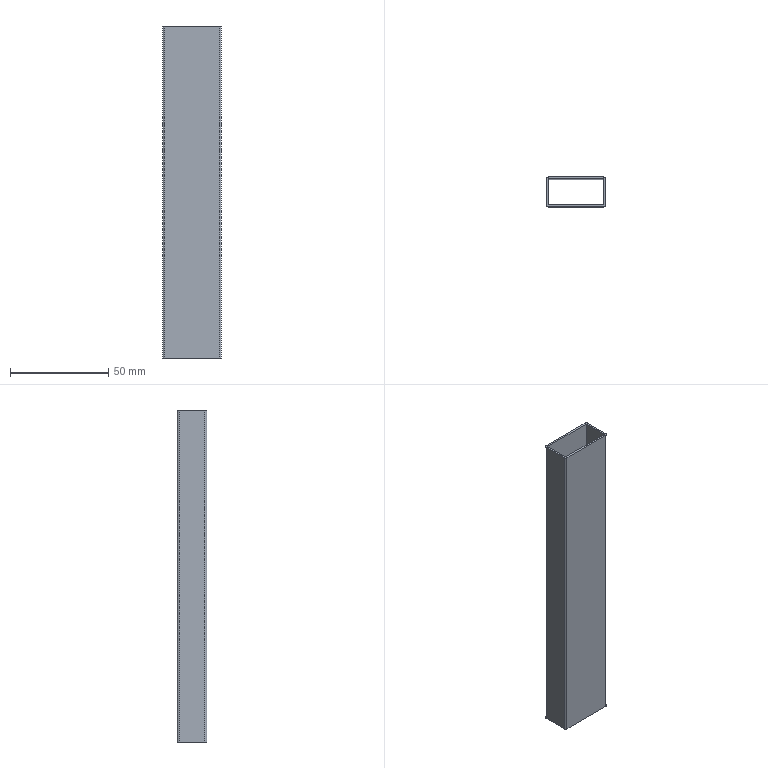Part | STEP file | Q7C1209 | 1 solid | 14 faces | box 30 x 15 x 169 mm | volume 14389 mm3 | plane 10 | cylinder 4 | commonest cylinder face diameters 2 x4
STEP:
#1=CARTESIAN_POINT('',(0.,0.,0.));
#2=DIRECTION('',(0.,0.,1.));
#3=DIRECTION('',(1.,0.,0.));
#4=AXIS2_PLACEMENT_3D('',#1,#2,#3);
#5=CARTESIAN_POINT('',(-14.,7.5,84.5));
#6=VERTEX_POINT('',#5);
#7=CARTESIAN_POINT('',(-15.,6.5,84.5));
#8=VERTEX_POINT('',#7);
#9=CARTESIAN_POINT('',(-14.,6.5,84.5));
#10=DIRECTION('',(0.,0.,1.));
#11=DIRECTION('',(1.,0.,0.));
#12=AXIS2_PLACEMENT_3D('',#9,#10,#11);
#13=CIRCLE('',#12,1.);
#14=CARTESIAN_POINT('',(-14.,6.5,84.5));
#15=DIRECTION('',(0.,0.,1.));
#16=DIRECTION('',(1.,0.,0.));
#17=AXIS2_PLACEMENT_3D('',#14,#15,#16);
#18=PLANE('',#17);
#19=CARTESIAN_POINT('',(0.,0.));
#20=DIRECTION('',(1.,0.));
#21=AXIS2_PLACEMENT_2D('',#19,#20);
#22=CIRCLE('',#21,1.);
#23=(GEOMETRIC_REPRESENTATION_CONTEXT(2)PARAMETRIC_REPRESENTATION_CONTEXT()REPRESENTATION_CONTEXT('',''));
#24=DEFINITIONAL_REPRESENTATION('',(#22),#23);
#25=PCURVE('',#18,#24);
#26=CARTESIAN_POINT('',(-14.,6.5,84.5));
#27=DIRECTION('',(0.,0.,-1.));
#28=DIRECTION('',(-1.,0.,0.));
#29=AXIS2_PLACEMENT_3D('',#26,#27,#28);
#30=CYLINDRICAL_SURFACE('',#29,1.);
#31=CARTESIAN_POINT('',(3.142,0.));
#32=DIRECTION('',(-1.,0.));
#33=VECTOR('',#32,1.);
#34=LINE('',#31,#33);
#35=(GEOMETRIC_REPRESENTATION_CONTEXT(2)PARAMETRIC_REPRESENTATION_CONTEXT()REPRESENTATION_CONTEXT('',''));
#36=DEFINITIONAL_REPRESENTATION('',(#34),#35);
#37=PCURVE('',#30,#36);
#38=SURFACE_CURVE('',#13,(#25,#37),.PCURVE_S1.);
#39=EDGE_CURVE('',#6,#8,#38,.T.);
#40=ORIENTED_EDGE('',*,*,#39,.T.);
#41=CARTESIAN_POINT('',(-15.,-6.5,84.5));
#42=VERTEX_POINT('',#41);
#43=CARTESIAN_POINT('',(-15.,6.5,84.5));
#44=DIRECTION('',(0.,-1.,0.));
#45=VECTOR('',#44,1.);
#46=LINE('',#43,#45);
#47=CARTESIAN_POINT('',(-1.,0.));
#48=DIRECTION('',(0.,-1.));
#49=VECTOR('',#48,1.);
#50=LINE('',#47,#49);
#51=(GEOMETRIC_REPRESENTATION_CONTEXT(2)PARAMETRIC_REPRESENTATION_CONTEXT()REPRESENTATION_CONTEXT('',''));
#52=DEFINITIONAL_REPRESENTATION('',(#50),#51);
#53=PCURVE('',#18,#52);
#54=CARTESIAN_POINT('',(-15.,6.5,84.5));
#55=DIRECTION('',(1.,0.,0.));
#56=DIRECTION('',(0.,1.,0.));
#57=AXIS2_PLACEMENT_3D('',#54,#55,#56);
#58=PLANE('',#57);
#59=CARTESIAN_POINT('',(0.,0.));
#60=DIRECTION('',(-1.,0.));
#61=VECTOR('',#60,1.);
#62=LINE('',#59,#61);
#63=(GEOMETRIC_REPRESENTATION_CONTEXT(2)PARAMETRIC_REPRESENTATION_CONTEXT()REPRESENTATION_CONTEXT('',''));
#64=DEFINITIONAL_REPRESENTATION('',(#62),#63);
#65=PCURVE('',#58,#64);
#66=SURFACE_CURVE('',#46,(#53,#65),.PCURVE_S1.);
#67=EDGE_CURVE('',#8,#42,#66,.T.);
#68=ORIENTED_EDGE('',*,*,#67,.T.);
#69=CARTESIAN_POINT('',(-14.,-7.5,84.5));
#70=VERTEX_POINT('',#69);
#71=CARTESIAN_POINT('',(-14.,-6.5,84.5));
#72=DIRECTION('',(0.,0.,1.));
#73=DIRECTION('',(1.,0.,0.));
#74=AXIS2_PLACEMENT_3D('',#71,#72,#73);
#75=CIRCLE('',#74,1.);
#76=CARTESIAN_POINT('',(0.,-13.));
#77=DIRECTION('',(1.,0.));
#78=AXIS2_PLACEMENT_2D('',#76,#77);
#79=CIRCLE('',#78,1.);
#80=(GEOMETRIC_REPRESENTATION_CONTEXT(2)PARAMETRIC_REPRESENTATION_CONTEXT()REPRESENTATION_CONTEXT('',''));
#81=DEFINITIONAL_REPRESENTATION('',(#79),#80);
#82=PCURVE('',#18,#81);
#83=CARTESIAN_POINT('',(-14.,-6.5,84.5));
#84=DIRECTION('',(0.,0.,-1.));
#85=DIRECTION('',(-1.,0.,0.));
#86=AXIS2_PLACEMENT_3D('',#83,#84,#85);
#87=CYLINDRICAL_SURFACE('',#86,1.);
#88=CARTESIAN_POINT('',(9.425,0.));
#89=DIRECTION('',(-1.,0.));
#90=VECTOR('',#89,1.);
#91=LINE('',#88,#90);
#92=(GEOMETRIC_REPRESENTATION_CONTEXT(2)PARAMETRIC_REPRESENTATION_CONTEXT()REPRESENTATION_CONTEXT('',''));
#93=DEFINITIONAL_REPRESENTATION('',(#91),#92);
#94=PCURVE('',#87,#93);
#95=SURFACE_CURVE('',#75,(#82,#94),.PCURVE_S1.);
#96=EDGE_CURVE('',#42,#70,#95,.T.);
#97=ORIENTED_EDGE('',*,*,#96,.T.);
#98=CARTESIAN_POINT('',(14.,-7.5,84.5));
#99=VERTEX_POINT('',#98);
#100=CARTESIAN_POINT('',(-14.,-7.5,84.5));
#101=DIRECTION('',(1.,0.,0.));
#102=VECTOR('',#101,1.);
#103=LINE('',#100,#102);
#104=CARTESIAN_POINT('',(0.,-14.));
#105=DIRECTION('',(1.,0.));
#106=VECTOR('',#105,1.);
#107=LINE('',#104,#106);
#108=(GEOMETRIC_REPRESENTATION_CONTEXT(2)PARAMETRIC_REPRESENTATION_CONTEXT()REPRESENTATION_CONTEXT('',''));
#109=DEFINITIONAL_REPRESENTATION('',(#107),#108);
#110=PCURVE('',#18,#109);
#111=CARTESIAN_POINT('',(-14.,-7.5,84.5));
#112=DIRECTION('',(0.,1.,0.));
#113=DIRECTION('',(0.,0.,1.));
#114=AXIS2_PLACEMENT_3D('',#111,#112,#113);
#115=PLANE('',#114);
#116=CARTESIAN_POINT('',(0.,0.));
#117=DIRECTION('',(0.,1.));
#118=VECTOR('',#117,1.);
#119=LINE('',#116,#118);
#120=(GEOMETRIC_REPRESENTATION_CONTEXT(2)PARAMETRIC_REPRESENTATION_CONTEXT()REPRESENTATION_CONTEXT('',''));
#121=DEFINITIONAL_REPRESENTATION('',(#119),#120);
#122=PCURVE('',#115,#121);
#123=SURFACE_CURVE('',#103,(#110,#122),.PCURVE_S1.);
#124=EDGE_CURVE('',#70,#99,#123,.T.);
#125=ORIENTED_EDGE('',*,*,#124,.T.);
#126=CARTESIAN_POINT('',(15.,-6.5,84.5));
#127=VERTEX_POINT('',#126);
#128=CARTESIAN_POINT('',(14.,-6.5,84.5));
#129=DIRECTION('',(0.,0.,1.));
#130=DIRECTION('',(1.,0.,0.));
#131=AXIS2_PLACEMENT_3D('',#128,#129,#130);
#132=CIRCLE('',#131,1.);
#133=CARTESIAN_POINT('',(28.,-13.));
#134=DIRECTION('',(1.,0.));
#135=AXIS2_PLACEMENT_2D('',#133,#134);
#136=CIRCLE('',#135,1.);
#137=(GEOMETRIC_REPRESENTATION_CONTEXT(2)PARAMETRIC_REPRESENTATION_CONTEXT()REPRESENTATION_CONTEXT('',''));
#138=DEFINITIONAL_REPRESENTATION('',(#136),#137);
#139=PCURVE('',#18,#138);
#140=CARTESIAN_POINT('',(14.,-6.5,84.5));
#141=DIRECTION('',(0.,0.,-1.));
#142=DIRECTION('',(-1.,0.,0.));
#143=AXIS2_PLACEMENT_3D('',#140,#141,#142);
#144=CYLINDRICAL_SURFACE('',#143,1.);
#145=CARTESIAN_POINT('',(9.425,0.));
#146=DIRECTION('',(-1.,0.));
#147=VECTOR('',#146,1.);
#148=LINE('',#145,#147);
#149=(GEOMETRIC_REPRESENTATION_CONTEXT(2)PARAMETRIC_REPRESENTATION_CONTEXT()REPRESENTATION_CONTEXT('',''));
#150=DEFINITIONAL_REPRESENTATION('',(#148),#149);
#151=PCURVE('',#144,#150);
#152=SURFACE_CURVE('',#132,(#139,#151),.PCURVE_S1.);
#153=EDGE_CURVE('',#99,#127,#152,.T.);
#154=ORIENTED_EDGE('',*,*,#153,.T.);
#155=CARTESIAN_POINT('',(15.,6.5,84.5));
#156=VERTEX_POINT('',#155);
#157=CARTESIAN_POINT('',(15.,6.5,84.5));
#158=DIRECTION('',(0.,1.,0.));
#159=VECTOR('',#158,1.);
#160=LINE('',#157,#159);
#161=CARTESIAN_POINT('',(29.,0.));
#162=DIRECTION('',(0.,1.));
#163=VECTOR('',#162,1.);
#164=LINE('',#161,#163);
#165=(GEOMETRIC_REPRESENTATION_CONTEXT(2)PARAMETRIC_REPRESENTATION_CONTEXT()REPRESENTATION_CONTEXT('',''));
#166=DEFINITIONAL_REPRESENTATION('',(#164),#165);
#167=PCURVE('',#18,#166);
#168=CARTESIAN_POINT('',(15.,6.5,84.5));
#169=DIRECTION('',(-1.,0.,0.));
#170=DIRECTION('',(0.,-1.,0.));
#171=AXIS2_PLACEMENT_3D('',#168,#169,#170);
#172=PLANE('',#171);
#173=CARTESIAN_POINT('',(0.,0.));
#174=DIRECTION('',(-1.,0.));
#175=VECTOR('',#174,1.);
#176=LINE('',#173,#175);
#177=(GEOMETRIC_REPRESENTATION_CONTEXT(2)PARAMETRIC_REPRESENTATION_CONTEXT()REPRESENTATION_CONTEXT('',''));
#178=DEFINITIONAL_REPRESENTATION('',(#176),#177);
#179=PCURVE('',#172,#178);
#180=SURFACE_CURVE('',#160,(#167,#179),.PCURVE_S1.);
#181=EDGE_CURVE('',#127,#156,#180,.T.);
#182=ORIENTED_EDGE('',*,*,#181,.T.);
#183=CARTESIAN_POINT('',(14.,7.5,84.5));
#184=VERTEX_POINT('',#183);
#185=CARTESIAN_POINT('',(14.,6.5,84.5));
#186=DIRECTION('',(0.,0.,1.));
#187=DIRECTION('',(-1.,0.,0.));
#188=AXIS2_PLACEMENT_3D('',#185,#186,#187);
#189=CIRCLE('',#188,1.);
#190=CARTESIAN_POINT('',(28.,0.));
#191=DIRECTION('',(-1.,0.));
#192=AXIS2_PLACEMENT_2D('',#190,#191);
#193=CIRCLE('',#192,1.);
#194=(GEOMETRIC_REPRESENTATION_CONTEXT(2)PARAMETRIC_REPRESENTATION_CONTEXT()REPRESENTATION_CONTEXT('',''));
#195=DEFINITIONAL_REPRESENTATION('',(#193),#194);
#196=PCURVE('',#18,#195);
#197=CARTESIAN_POINT('',(14.,6.5,84.5));
#198=DIRECTION('',(0.,0.,-1.));
#199=DIRECTION('',(-1.,0.,0.));
#200=AXIS2_PLACEMENT_3D('',#197,#198,#199);
#201=CYLINDRICAL_SURFACE('',#200,1.);
#202=CARTESIAN_POINT('',(6.283,0.));
#203=DIRECTION('',(-1.,0.));
#204=VECTOR('',#203,1.);
#205=LINE('',#202,#204);
#206=(GEOMETRIC_REPRESENTATION_CONTEXT(2)PARAMETRIC_REPRESENTATION_CONTEXT()REPRESENTATION_CONTEXT('',''));
#207=DEFINITIONAL_REPRESENTATION('',(#205),#206);
#208=PCURVE('',#201,#207);
#209=SURFACE_CURVE('',#189,(#196,#208),.PCURVE_S1.);
#210=EDGE_CURVE('',#156,#184,#209,.T.);
#211=ORIENTED_EDGE('',*,*,#210,.T.);
#212=CARTESIAN_POINT('',(-14.,7.5,84.5));
#213=DIRECTION('',(-1.,0.,0.));
#214=VECTOR('',#213,1.);
#215=LINE('',#212,#214);
#216=CARTESIAN_POINT('',(0.,1.));
#217=DIRECTION('',(-1.,0.));
#218=VECTOR('',#217,1.);
#219=LINE('',#216,#218);
#220=(GEOMETRIC_REPRESENTATION_CONTEXT(2)PARAMETRIC_REPRESENTATION_CONTEXT()REPRESENTATION_CONTEXT('',''));
#221=DEFINITIONAL_REPRESENTATION('',(#219),#220);
#222=PCURVE('',#18,#221);
#223=CARTESIAN_POINT('',(-14.,7.5,84.5));
#224=DIRECTION('',(0.,-1.,0.));
#225=DIRECTION('',(0.,0.,-1.));
#226=AXIS2_PLACEMENT_3D('',#223,#224,#225);
#227=PLANE('',#226);
#228=CARTESIAN_POINT('',(0.,0.));
#229=DIRECTION('',(0.,-1.));
#230=VECTOR('',#229,1.);
#231=LINE('',#228,#230);
#232=(GEOMETRIC_REPRESENTATION_CONTEXT(2)PARAMETRIC_REPRESENTATION_CONTEXT()REPRESENTATION_CONTEXT('',''));
#233=DEFINITIONAL_REPRESENTATION('',(#231),#232);
#234=PCURVE('',#227,#233);
#235=SURFACE_CURVE('',#215,(#222,#234),.PCURVE_S1.);
#236=EDGE_CURVE('',#184,#6,#235,.T.);
#237=ORIENTED_EDGE('',*,*,#236,.T.);
#238=EDGE_LOOP('',(#40,#68,#97,#125,#154,#182,#211,#237));
#239=FACE_BOUND('',#238,.T.);
#240=CARTESIAN_POINT('',(-14.,6.5,84.5));
#241=VERTEX_POINT('',#240);
#242=CARTESIAN_POINT('',(-14.,-6.5,84.5));
#243=VERTEX_POINT('',#242);
#244=CARTESIAN_POINT('',(-14.,6.5,84.5));
#245=DIRECTION('',(0.,-1.,0.));
#246=VECTOR('',#245,1.);
#247=LINE('',#244,#246);
#248=CARTESIAN_POINT('',(0.,0.));
#249=DIRECTION('',(0.,-1.));
#250=VECTOR('',#249,1.);
#251=LINE('',#248,#250);
#252=(GEOMETRIC_REPRESENTATION_CONTEXT(2)PARAMETRIC_REPRESENTATION_CONTEXT()REPRESENTATION_CONTEXT('',''));
#253=DEFINITIONAL_REPRESENTATION('',(#251),#252);
#254=PCURVE('',#18,#253);
#255=CARTESIAN_POINT('',(-14.,6.5,84.5));
#256=DIRECTION('',(1.,0.,0.));
#257=DIRECTION('',(0.,1.,0.));
#258=AXIS2_PLACEMENT_3D('',#255,#256,#257);
#259=PLANE('',#258);
#260=CARTESIAN_POINT('',(0.,0.));
#261=DIRECTION('',(-1.,0.));
#262=VECTOR('',#261,1.);
#263=LINE('',#260,#262);
#264=(GEOMETRIC_REPRESENTATION_CONTEXT(2)PARAMETRIC_REPRESENTATION_CONTEXT()REPRESENTATION_CONTEXT('',''));
#265=DEFINITIONAL_REPRESENTATION('',(#263),#264);
#266=PCURVE('',#259,#265);
#267=SURFACE_CURVE('',#247,(#254,#266),.PCURVE_S1.);
#268=EDGE_CURVE('',#241,#243,#267,.T.);
#269=ORIENTED_EDGE('',*,*,#268,.F.);
#270=CARTESIAN_POINT('',(14.,6.5,84.5));
#271=VERTEX_POINT('',#270);
#272=CARTESIAN_POINT('',(-14.,6.5,84.5));
#273=DIRECTION('',(-1.,0.,0.));
#274=VECTOR('',#273,1.);
#275=LINE('',#272,#274);
#276=CARTESIAN_POINT('',(0.,0.));
#277=DIRECTION('',(-1.,0.));
#278=VECTOR('',#277,1.);
#279=LINE('',#276,#278);
#280=(GEOMETRIC_REPRESENTATION_CONTEXT(2)PARAMETRIC_REPRESENTATION_CONTEXT()REPRESENTATION_CONTEXT('',''));
#281=DEFINITIONAL_REPRESENTATION('',(#279),#280);
#282=PCURVE('',#18,#281);
#283=CARTESIAN_POINT('',(-14.,6.5,84.5));
#284=DIRECTION('',(0.,-1.,0.));
#285=DIRECTION('',(0.,0.,-1.));
#286=AXIS2_PLACEMENT_3D('',#283,#284,#285);
#287=PLANE('',#286);
#288=CARTESIAN_POINT('',(0.,0.));
#289=DIRECTION('',(0.,-1.));
#290=VECTOR('',#289,1.);
#291=LINE('',#288,#290);
#292=(GEOMETRIC_REPRESENTATION_CONTEXT(2)PARAMETRIC_REPRESENTATION_CONTEXT()REPRESENTATION_CONTEXT('',''));
#293=DEFINITIONAL_REPRESENTATION('',(#291),#292);
#294=PCURVE('',#287,#293);
#295=SURFACE_CURVE('',#275,(#282,#294),.PCURVE_S1.);
#296=EDGE_CURVE('',#271,#241,#295,.T.);
#297=ORIENTED_EDGE('',*,*,#296,.F.);
#298=CARTESIAN_POINT('',(14.,-6.5,84.5));
#299=VERTEX_POINT('',#298);
#300=CARTESIAN_POINT('',(14.,6.5,84.5));
#301=DIRECTION('',(0.,1.,0.));
#302=VECTOR('',#301,1.);
#303=LINE('',#300,#302);
#304=CARTESIAN_POINT('',(28.,0.));
#305=DIRECTION('',(0.,1.));
#306=VECTOR('',#305,1.);
#307=LINE('',#304,#306);
#308=(GEOMETRIC_REPRESENTATION_CONTEXT(2)PARAMETRIC_REPRESENTATION_CONTEXT()REPRESENTATION_CONTEXT('',''));
#309=DEFINITIONAL_REPRESENTATION('',(#307),#308);
#310=PCURVE('',#18,#309);
#311=CARTESIAN_POINT('',(14.,6.5,84.5));
#312=DIRECTION('',(-1.,0.,0.));
#313=DIRECTION('',(0.,-1.,0.));
#314=AXIS2_PLACEMENT_3D('',#311,#312,#313);
#315=PLANE('',#314);
#316=CARTESIAN_POINT('',(0.,0.));
#317=DIRECTION('',(-1.,0.));
#318=VECTOR('',#317,1.);
#319=LINE('',#316,#318);
#320=(GEOMETRIC_REPRESENTATION_CONTEXT(2)PARAMETRIC_REPRESENTATION_CONTEXT()REPRESENTATION_CONTEXT('',''));
#321=DEFINITIONAL_REPRESENTATION('',(#319),#320);
#322=PCURVE('',#315,#321);
#323=SURFACE_CURVE('',#303,(#310,#322),.PCURVE_S1.);
#324=EDGE_CURVE('',#299,#271,#323,.T.);
#325=ORIENTED_EDGE('',*,*,#324,.F.);
#326=CARTESIAN_POINT('',(-14.,-6.5,84.5));
#327=DIRECTION('',(1.,0.,0.));
#328=VECTOR('',#327,1.);
#329=LINE('',#326,#328);
#330=CARTESIAN_POINT('',(0.,-13.));
#331=DIRECTION('',(1.,0.));
#332=VECTOR('',#331,1.);
#333=LINE('',#330,#332);
#334=(GEOMETRIC_REPRESENTATION_CONTEXT(2)PARAMETRIC_REPRESENTATION_CONTEXT()REPRESENTATION_CONTEXT('',''));
#335=DEFINITIONAL_REPRESENTATION('',(#333),#334);
#336=PCURVE('',#18,#335);
#337=CARTESIAN_POINT('',(-14.,-6.5,84.5));
#338=DIRECTION('',(0.,1.,0.));
#339=DIRECTION('',(0.,0.,1.));
#340=AXIS2_PLACEMENT_3D('',#337,#338,#339);
#341=PLANE('',#340);
#342=CARTESIAN_POINT('',(0.,0.));
#343=DIRECTION('',(0.,1.));
#344=VECTOR('',#343,1.);
#345=LINE('',#342,#344);
#346=(GEOMETRIC_REPRESENTATION_CONTEXT(2)PARAMETRIC_REPRESENTATION_CONTEXT()REPRESENTATION_CONTEXT('',''));
#347=DEFINITIONAL_REPRESENTATION('',(#345),#346);
#348=PCURVE('',#341,#347);
#349=SURFACE_CURVE('',#329,(#336,#348),.PCURVE_S1.);
#350=EDGE_CURVE('',#243,#299,#349,.T.);
#351=ORIENTED_EDGE('',*,*,#350,.F.);
#352=EDGE_LOOP('',(#269,#297,#325,#351));
#353=FACE_BOUND('',#352,.T.);
#354=ADVANCED_FACE('',(#239,#353),#18,.T.);
#355=CARTESIAN_POINT('',(-14.,7.5,-84.5));
#356=VERTEX_POINT('',#355);
#357=CARTESIAN_POINT('',(-15.,6.5,-84.5));
#358=VERTEX_POINT('',#357);
#359=CARTESIAN_POINT('',(-14.,6.5,-84.5));
#360=DIRECTION('',(0.,0.,1.));
#361=DIRECTION('',(1.,0.,0.));
#362=AXIS2_PLACEMENT_3D('',#359,#360,#361);
#363=CIRCLE('',#362,1.);
#364=CARTESIAN_POINT('',(-14.,6.5,-84.5));
#365=DIRECTION('',(0.,0.,1.));
#366=DIRECTION('',(1.,0.,0.));
#367=AXIS2_PLACEMENT_3D('',#364,#365,#366);
#368=PLANE('',#367);
#369=CARTESIAN_POINT('',(0.,0.));
#370=DIRECTION('',(1.,0.));
#371=AXIS2_PLACEMENT_2D('',#369,#370);
#372=CIRCLE('',#371,1.);
#373=(GEOMETRIC_REPRESENTATION_CONTEXT(2)PARAMETRIC_REPRESENTATION_CONTEXT()REPRESENTATION_CONTEXT('',''));
#374=DEFINITIONAL_REPRESENTATION('',(#372),#373);
#375=PCURVE('',#368,#374);
#376=CARTESIAN_POINT('',(3.142,169.));
#377=DIRECTION('',(-1.,0.));
#378=VECTOR('',#377,1.);
#379=LINE('',#376,#378);
#380=(GEOMETRIC_REPRESENTATION_CONTEXT(2)PARAMETRIC_REPRESENTATION_CONTEXT()REPRESENTATION_CONTEXT('',''));
#381=DEFINITIONAL_REPRESENTATION('',(#379),#380);
#382=PCURVE('',#30,#381);
#383=SURFACE_CURVE('',#363,(#375,#382),.PCURVE_S1.);
#384=EDGE_CURVE('',#356,#358,#383,.T.);
#385=ORIENTED_EDGE('',*,*,#384,.F.);
#386=CARTESIAN_POINT('',(14.,7.5,-84.5));
#387=VERTEX_POINT('',#386);
#388=CARTESIAN_POINT('',(-14.,7.5,-84.5));
#389=DIRECTION('',(-1.,0.,0.));
#390=VECTOR('',#389,1.);
#391=LINE('',#388,#390);
#392=CARTESIAN_POINT('',(0.,1.));
#393=DIRECTION('',(-1.,0.));
#394=VECTOR('',#393,1.);
#395=LINE('',#392,#394);
#396=(GEOMETRIC_REPRESENTATION_CONTEXT(2)PARAMETRIC_REPRESENTATION_CONTEXT()REPRESENTATION_CONTEXT('',''));
#397=DEFINITIONAL_REPRESENTATION('',(#395),#396);
#398=PCURVE('',#368,#397);
#399=CARTESIAN_POINT('',(169.,0.));
#400=DIRECTION('',(0.,-1.));
#401=VECTOR('',#400,1.);
#402=LINE('',#399,#401);
#403=(GEOMETRIC_REPRESENTATION_CONTEXT(2)PARAMETRIC_REPRESENTATION_CONTEXT()REPRESENTATION_CONTEXT('',''));
#404=DEFINITIONAL_REPRESENTATION('',(#402),#403);
#405=PCURVE('',#227,#404);
#406=SURFACE_CURVE('',#391,(#398,#405),.PCURVE_S1.);
#407=EDGE_CURVE('',#387,#356,#406,.T.);
#408=ORIENTED_EDGE('',*,*,#407,.F.);
#409=CARTESIAN_POINT('',(15.,6.5,-84.5));
#410=VERTEX_POINT('',#409);
#411=CARTESIAN_POINT('',(14.,6.5,-84.5));
#412=DIRECTION('',(0.,0.,1.));
#413=DIRECTION('',(-1.,0.,0.));
#414=AXIS2_PLACEMENT_3D('',#411,#412,#413);
#415=CIRCLE('',#414,1.);
#416=CARTESIAN_POINT('',(28.,0.));
#417=DIRECTION('',(-1.,0.));
#418=AXIS2_PLACEMENT_2D('',#416,#417);
#419=CIRCLE('',#418,1.);
#420=(GEOMETRIC_REPRESENTATION_CONTEXT(2)PARAMETRIC_REPRESENTATION_CONTEXT()REPRESENTATION_CONTEXT('',''));
#421=DEFINITIONAL_REPRESENTATION('',(#419),#420);
#422=PCURVE('',#368,#421);
#423=CARTESIAN_POINT('',(6.283,169.));
#424=DIRECTION('',(-1.,0.));
#425=VECTOR('',#424,1.);
#426=LINE('',#423,#425);
#427=(GEOMETRIC_REPRESENTATION_CONTEXT(2)PARAMETRIC_REPRESENTATION_CONTEXT()REPRESENTATION_CONTEXT('',''));
#428=DEFINITIONAL_REPRESENTATION('',(#426),#427);
#429=PCURVE('',#201,#428);
#430=SURFACE_CURVE('',#415,(#422,#429),.PCURVE_S1.);
#431=EDGE_CURVE('',#410,#387,#430,.T.);
#432=ORIENTED_EDGE('',*,*,#431,.F.);
#433=CARTESIAN_POINT('',(15.,-6.5,-84.5));
#434=VERTEX_POINT('',#433);
#435=CARTESIAN_POINT('',(15.,6.5,-84.5));
#436=DIRECTION('',(0.,1.,0.));
#437=VECTOR('',#436,1.);
#438=LINE('',#435,#437);
#439=CARTESIAN_POINT('',(29.,0.));
#440=DIRECTION('',(0.,1.));
#441=VECTOR('',#440,1.);
#442=LINE('',#439,#441);
#443=(GEOMETRIC_REPRESENTATION_CONTEXT(2)PARAMETRIC_REPRESENTATION_CONTEXT()REPRESENTATION_CONTEXT('',''));
#444=DEFINITIONAL_REPRESENTATION('',(#442),#443);
#445=PCURVE('',#368,#444);
#446=CARTESIAN_POINT('',(0.,-169.));
#447=DIRECTION('',(-1.,0.));
#448=VECTOR('',#447,1.);
#449=LINE('',#446,#448);
#450=(GEOMETRIC_REPRESENTATION_CONTEXT(2)PARAMETRIC_REPRESENTATION_CONTEXT()REPRESENTATION_CONTEXT('',''));
#451=DEFINITIONAL_REPRESENTATION('',(#449),#450);
#452=PCURVE('',#172,#451);
#453=SURFACE_CURVE('',#438,(#445,#452),.PCURVE_S1.);
#454=EDGE_CURVE('',#434,#410,#453,.T.);
#455=ORIENTED_EDGE('',*,*,#454,.F.);
#456=CARTESIAN_POINT('',(14.,-7.5,-84.5));
#457=VERTEX_POINT('',#456);
#458=CARTESIAN_POINT('',(14.,-6.5,-84.5));
#459=DIRECTION('',(0.,0.,1.));
#460=DIRECTION('',(1.,0.,0.));
#461=AXIS2_PLACEMENT_3D('',#458,#459,#460);
#462=CIRCLE('',#461,1.);
#463=CARTESIAN_POINT('',(28.,-13.));
#464=DIRECTION('',(1.,0.));
#465=AXIS2_PLACEMENT_2D('',#463,#464);
#466=CIRCLE('',#465,1.);
#467=(GEOMETRIC_REPRESENTATION_CONTEXT(2)PARAMETRIC_REPRESENTATION_CONTEXT()REPRESENTATION_CONTEXT('',''));
#468=DEFINITIONAL_REPRESENTATION('',(#466),#467);
#469=PCURVE('',#368,#468);
#470=CARTESIAN_POINT('',(9.425,169.));
#471=DIRECTION('',(-1.,0.));
#472=VECTOR('',#471,1.);
#473=LINE('',#470,#472);
#474=(GEOMETRIC_REPRESENTATION_CONTEXT(2)PARAMETRIC_REPRESENTATION_CONTEXT()REPRESENTATION_CONTEXT('',''));
#475=DEFINITIONAL_REPRESENTATION('',(#473),#474);
#476=PCURVE('',#144,#475);
#477=SURFACE_CURVE('',#462,(#469,#476),.PCURVE_S1.);
#478=EDGE_CURVE('',#457,#434,#477,.T.);
#479=ORIENTED_EDGE('',*,*,#478,.F.);
#480=CARTESIAN_POINT('',(-14.,-7.5,-84.5));
#481=VERTEX_POINT('',#480);
#482=CARTESIAN_POINT('',(-14.,-7.5,-84.5));
#483=DIRECTION('',(1.,0.,0.));
#484=VECTOR('',#483,1.);
#485=LINE('',#482,#484);
#486=CARTESIAN_POINT('',(0.,-14.));
#487=DIRECTION('',(1.,0.));
#488=VECTOR('',#487,1.);
#489=LINE('',#486,#488);
#490=(GEOMETRIC_REPRESENTATION_CONTEXT(2)PARAMETRIC_REPRESENTATION_CONTEXT()REPRESENTATION_CONTEXT('',''));
#491=DEFINITIONAL_REPRESENTATION('',(#489),#490);
#492=PCURVE('',#368,#491);
#493=CARTESIAN_POINT('',(-169.,0.));
#494=DIRECTION('',(0.,1.));
#495=VECTOR('',#494,1.);
#496=LINE('',#493,#495);
#497=(GEOMETRIC_REPRESENTATION_CONTEXT(2)PARAMETRIC_REPRESENTATION_CONTEXT()REPRESENTATION_CONTEXT('',''));
#498=DEFINITIONAL_REPRESENTATION('',(#496),#497);
#499=PCURVE('',#115,#498);
#500=SURFACE_CURVE('',#485,(#492,#499),.PCURVE_S1.);
#501=EDGE_CURVE('',#481,#457,#500,.T.);
#502=ORIENTED_EDGE('',*,*,#501,.F.);
#503=CARTESIAN_POINT('',(-15.,-6.5,-84.5));
#504=VERTEX_POINT('',#503);
#505=CARTESIAN_POINT('',(-14.,-6.5,-84.5));
#506=DIRECTION('',(0.,0.,1.));
#507=DIRECTION('',(1.,0.,0.));
#508=AXIS2_PLACEMENT_3D('',#505,#506,#507);
#509=CIRCLE('',#508,1.);
#510=CARTESIAN_POINT('',(0.,-13.));
#511=DIRECTION('',(1.,0.));
#512=AXIS2_PLACEMENT_2D('',#510,#511);
#513=CIRCLE('',#512,1.);
#514=(GEOMETRIC_REPRESENTATION_CONTEXT(2)PARAMETRIC_REPRESENTATION_CONTEXT()REPRESENTATION_CONTEXT('',''));
#515=DEFINITIONAL_REPRESENTATION('',(#513),#514);
#516=PCURVE('',#368,#515);
#517=CARTESIAN_POINT('',(9.425,169.));
#518=DIRECTION('',(-1.,0.));
#519=VECTOR('',#518,1.);
#520=LINE('',#517,#519);
#521=(GEOMETRIC_REPRESENTATION_CONTEXT(2)PARAMETRIC_REPRESENTATION_CONTEXT()REPRESENTATION_CONTEXT('',''));
#522=DEFINITIONAL_REPRESENTATION('',(#520),#521);
#523=PCURVE('',#87,#522);
#524=SURFACE_CURVE('',#509,(#516,#523),.PCURVE_S1.);
#525=EDGE_CURVE('',#504,#481,#524,.T.);
#526=ORIENTED_EDGE('',*,*,#525,.F.);
#527=CARTESIAN_POINT('',(-15.,6.5,-84.5));
#528=DIRECTION('',(0.,-1.,0.));
#529=VECTOR('',#528,1.);
#530=LINE('',#527,#529);
#531=CARTESIAN_POINT('',(-1.,0.));
#532=DIRECTION('',(0.,-1.));
#533=VECTOR('',#532,1.);
#534=LINE('',#531,#533);
#535=(GEOMETRIC_REPRESENTATION_CONTEXT(2)PARAMETRIC_REPRESENTATION_CONTEXT()REPRESENTATION_CONTEXT('',''));
#536=DEFINITIONAL_REPRESENTATION('',(#534),#535);
#537=PCURVE('',#368,#536);
#538=CARTESIAN_POINT('',(0.,-169.));
#539=DIRECTION('',(-1.,0.));
#540=VECTOR('',#539,1.);
#541=LINE('',#538,#540);
#542=(GEOMETRIC_REPRESENTATION_CONTEXT(2)PARAMETRIC_REPRESENTATION_CONTEXT()REPRESENTATION_CONTEXT('',''));
#543=DEFINITIONAL_REPRESENTATION('',(#541),#542);
#544=PCURVE('',#58,#543);
#545=SURFACE_CURVE('',#530,(#537,#544),.PCURVE_S1.);
#546=EDGE_CURVE('',#358,#504,#545,.T.);
#547=ORIENTED_EDGE('',*,*,#546,.F.);
#548=EDGE_LOOP('',(#385,#408,#432,#455,#479,#502,#526,#547));
#549=FACE_BOUND('',#548,.T.);
#550=CARTESIAN_POINT('',(14.,6.5,-84.5));
#551=VERTEX_POINT('',#550);
#552=CARTESIAN_POINT('',(-14.,6.5,-84.5));
#553=VERTEX_POINT('',#552);
#554=CARTESIAN_POINT('',(-14.,6.5,-84.5));
#555=DIRECTION('',(-1.,0.,0.));
#556=VECTOR('',#555,1.);
#557=LINE('',#554,#556);
#558=CARTESIAN_POINT('',(0.,0.));
#559=DIRECTION('',(-1.,0.));
#560=VECTOR('',#559,1.);
#561=LINE('',#558,#560);
#562=(GEOMETRIC_REPRESENTATION_CONTEXT(2)PARAMETRIC_REPRESENTATION_CONTEXT()REPRESENTATION_CONTEXT('',''));
#563=DEFINITIONAL_REPRESENTATION('',(#561),#562);
#564=PCURVE('',#368,#563);
#565=CARTESIAN_POINT('',(169.,0.));
#566=DIRECTION('',(0.,-1.));
#567=VECTOR('',#566,1.);
#568=LINE('',#565,#567);
#569=(GEOMETRIC_REPRESENTATION_CONTEXT(2)PARAMETRIC_REPRESENTATION_CONTEXT()REPRESENTATION_CONTEXT('',''));
#570=DEFINITIONAL_REPRESENTATION('',(#568),#569);
#571=PCURVE('',#287,#570);
#572=SURFACE_CURVE('',#557,(#564,#571),.PCURVE_S1.);
#573=EDGE_CURVE('',#551,#553,#572,.T.);
#574=ORIENTED_EDGE('',*,*,#573,.T.);
#575=CARTESIAN_POINT('',(-14.,-6.5,-84.5));
#576=VERTEX_POINT('',#575);
#577=CARTESIAN_POINT('',(-14.,6.5,-84.5));
#578=DIRECTION('',(0.,-1.,0.));
#579=VECTOR('',#578,1.);
#580=LINE('',#577,#579);
#581=CARTESIAN_POINT('',(0.,0.));
#582=DIRECTION('',(0.,-1.));
#583=VECTOR('',#582,1.);
#584=LINE('',#581,#583);
#585=(GEOMETRIC_REPRESENTATION_CONTEXT(2)PARAMETRIC_REPRESENTATION_CONTEXT()REPRESENTATION_CONTEXT('',''));
#586=DEFINITIONAL_REPRESENTATION('',(#584),#585);
#587=PCURVE('',#368,#586);
#588=CARTESIAN_POINT('',(0.,-169.));
#589=DIRECTION('',(-1.,0.));
#590=VECTOR('',#589,1.);
#591=LINE('',#588,#590);
#592=(GEOMETRIC_REPRESENTATION_CONTEXT(2)PARAMETRIC_REPRESENTATION_CONTEXT()REPRESENTATION_CONTEXT('',''));
#593=DEFINITIONAL_REPRESENTATION('',(#591),#592);
#594=PCURVE('',#259,#593);
#595=SURFACE_CURVE('',#580,(#587,#594),.PCURVE_S1.);
#596=EDGE_CURVE('',#553,#576,#595,.T.);
#597=ORIENTED_EDGE('',*,*,#596,.T.);
#598=CARTESIAN_POINT('',(14.,-6.5,-84.5));
#599=VERTEX_POINT('',#598);
#600=CARTESIAN_POINT('',(-14.,-6.5,-84.5));
#601=DIRECTION('',(1.,0.,0.));
#602=VECTOR('',#601,1.);
#603=LINE('',#600,#602);
#604=CARTESIAN_POINT('',(0.,-13.));
#605=DIRECTION('',(1.,0.));
#606=VECTOR('',#605,1.);
#607=LINE('',#604,#606);
#608=(GEOMETRIC_REPRESENTATION_CONTEXT(2)PARAMETRIC_REPRESENTATION_CONTEXT()REPRESENTATION_CONTEXT('',''));
#609=DEFINITIONAL_REPRESENTATION('',(#607),#608);
#610=PCURVE('',#368,#609);
#611=CARTESIAN_POINT('',(-169.,0.));
#612=DIRECTION('',(0.,1.));
#613=VECTOR('',#612,1.);
#614=LINE('',#611,#613);
#615=(GEOMETRIC_REPRESENTATION_CONTEXT(2)PARAMETRIC_REPRESENTATION_CONTEXT()REPRESENTATION_CONTEXT('',''));
#616=DEFINITIONAL_REPRESENTATION('',(#614),#615);
#617=PCURVE('',#341,#616);
#618=SURFACE_CURVE('',#603,(#610,#617),.PCURVE_S1.);
#619=EDGE_CURVE('',#576,#599,#618,.T.);
#620=ORIENTED_EDGE('',*,*,#619,.T.);
#621=CARTESIAN_POINT('',(14.,6.5,-84.5));
#622=DIRECTION('',(0.,1.,0.));
#623=VECTOR('',#622,1.);
#624=LINE('',#621,#623);
#625=CARTESIAN_POINT('',(28.,0.));
#626=DIRECTION('',(0.,1.));
#627=VECTOR('',#626,1.);
#628=LINE('',#625,#627);
#629=(GEOMETRIC_REPRESENTATION_CONTEXT(2)PARAMETRIC_REPRESENTATION_CONTEXT()REPRESENTATION_CONTEXT('',''));
#630=DEFINITIONAL_REPRESENTATION('',(#628),#629);
#631=PCURVE('',#368,#630);
#632=CARTESIAN_POINT('',(0.,-169.));
#633=DIRECTION('',(-1.,0.));
#634=VECTOR('',#633,1.);
#635=LINE('',#632,#634);
#636=(GEOMETRIC_REPRESENTATION_CONTEXT(2)PARAMETRIC_REPRESENTATION_CONTEXT()REPRESENTATION_CONTEXT('',''));
#637=DEFINITIONAL_REPRESENTATION('',(#635),#636);
#638=PCURVE('',#315,#637);
#639=SURFACE_CURVE('',#624,(#631,#638),.PCURVE_S1.);
#640=EDGE_CURVE('',#599,#551,#639,.T.);
#641=ORIENTED_EDGE('',*,*,#640,.T.);
#642=EDGE_LOOP('',(#574,#597,#620,#641));
#643=FACE_BOUND('',#642,.T.);
#644=ADVANCED_FACE('',(#549,#643),#368,.F.);
#645=ORIENTED_EDGE('',*,*,#384,.T.);
#646=CARTESIAN_POINT('',(-15.,6.5,84.5));
#647=DIRECTION('',(0.,0.,-1.));
#648=VECTOR('',#647,1.);
#649=LINE('',#646,#648);
#650=CARTESIAN_POINT('',(0.,0.));
#651=DIRECTION('',(0.,1.));
#652=VECTOR('',#651,1.);
#653=LINE('',#650,#652);
#654=(GEOMETRIC_REPRESENTATION_CONTEXT(2)PARAMETRIC_REPRESENTATION_CONTEXT()REPRESENTATION_CONTEXT('',''));
#655=DEFINITIONAL_REPRESENTATION('',(#653),#654);
#656=PCURVE('',#30,#655);
#657=CARTESIAN_POINT('',(0.,0.));
#658=DIRECTION('',(0.,-1.));
#659=VECTOR('',#658,1.);
#660=LINE('',#657,#659);
#661=(GEOMETRIC_REPRESENTATION_CONTEXT(2)PARAMETRIC_REPRESENTATION_CONTEXT()REPRESENTATION_CONTEXT('',''));
#662=DEFINITIONAL_REPRESENTATION('',(#660),#661);
#663=PCURVE('',#58,#662);
#664=SURFACE_CURVE('',#649,(#656,#663),.PCURVE_S1.);
#665=EDGE_CURVE('',#8,#358,#664,.T.);
#666=ORIENTED_EDGE('',*,*,#665,.F.);
#667=ORIENTED_EDGE('',*,*,#39,.F.);
#668=CARTESIAN_POINT('',(-14.,7.5,84.5));
#669=DIRECTION('',(0.,0.,-1.));
#670=VECTOR('',#669,1.);
#671=LINE('',#668,#670);
#672=CARTESIAN_POINT('',(1.571,0.));
#673=DIRECTION('',(0.,1.));
#674=VECTOR('',#673,1.);
#675=LINE('',#672,#674);
#676=(GEOMETRIC_REPRESENTATION_CONTEXT(2)PARAMETRIC_REPRESENTATION_CONTEXT()REPRESENTATION_CONTEXT('',''));
#677=DEFINITIONAL_REPRESENTATION('',(#675),#676);
#678=PCURVE('',#30,#677);
#679=CARTESIAN_POINT('',(0.,0.));
#680=DIRECTION('',(1.,0.));
#681=VECTOR('',#680,1.);
#682=LINE('',#679,#681);
#683=(GEOMETRIC_REPRESENTATION_CONTEXT(2)PARAMETRIC_REPRESENTATION_CONTEXT()REPRESENTATION_CONTEXT('',''));
#684=DEFINITIONAL_REPRESENTATION('',(#682),#683);
#685=PCURVE('',#227,#684);
#686=SURFACE_CURVE('',#671,(#678,#685),.PCURVE_S1.);
#687=EDGE_CURVE('',#6,#356,#686,.T.);
#688=ORIENTED_EDGE('',*,*,#687,.T.);
#689=EDGE_LOOP('',(#645,#666,#667,#688));
#690=FACE_BOUND('',#689,.T.);
#691=ADVANCED_FACE('',(#690),#30,.T.);
#692=ORIENTED_EDGE('',*,*,#546,.T.);
#693=CARTESIAN_POINT('',(-15.,-6.5,84.5));
#694=DIRECTION('',(0.,0.,-1.));
#695=VECTOR('',#694,1.);
#696=LINE('',#693,#695);
#697=CARTESIAN_POINT('',(-13.,0.));
#698=DIRECTION('',(0.,-1.));
#699=VECTOR('',#698,1.);
#700=LINE('',#697,#699);
#701=(GEOMETRIC_REPRESENTATION_CONTEXT(2)PARAMETRIC_REPRESENTATION_CONTEXT()REPRESENTATION_CONTEXT('',''));
#702=DEFINITIONAL_REPRESENTATION('',(#700),#701);
#703=PCURVE('',#58,#702);
#704=CARTESIAN_POINT('',(6.283,0.));
#705=DIRECTION('',(0.,1.));
#706=VECTOR('',#705,1.);
#707=LINE('',#704,#706);
#708=(GEOMETRIC_REPRESENTATION_CONTEXT(2)PARAMETRIC_REPRESENTATION_CONTEXT()REPRESENTATION_CONTEXT('',''));
#709=DEFINITIONAL_REPRESENTATION('',(#707),#708);
#710=PCURVE('',#87,#709);
#711=SURFACE_CURVE('',#696,(#703,#710),.PCURVE_S1.);
#712=EDGE_CURVE('',#42,#504,#711,.T.);
#713=ORIENTED_EDGE('',*,*,#712,.F.);
#714=ORIENTED_EDGE('',*,*,#67,.F.);
#715=ORIENTED_EDGE('',*,*,#665,.T.);
#716=EDGE_LOOP('',(#692,#713,#714,#715));
#717=FACE_BOUND('',#716,.T.);
#718=ADVANCED_FACE('',(#717),#58,.F.);
#719=ORIENTED_EDGE('',*,*,#525,.T.);
#720=CARTESIAN_POINT('',(-14.,-7.5,84.5));
#721=DIRECTION('',(0.,0.,-1.));
#722=VECTOR('',#721,1.);
#723=LINE('',#720,#722);
#724=CARTESIAN_POINT('',(4.712,0.));
#725=DIRECTION('',(0.,1.));
#726=VECTOR('',#725,1.);
#727=LINE('',#724,#726);
#728=(GEOMETRIC_REPRESENTATION_CONTEXT(2)PARAMETRIC_REPRESENTATION_CONTEXT()REPRESENTATION_CONTEXT('',''));
#729=DEFINITIONAL_REPRESENTATION('',(#727),#728);
#730=PCURVE('',#87,#729);
#731=CARTESIAN_POINT('',(0.,0.));
#732=DIRECTION('',(-1.,0.));
#733=VECTOR('',#732,1.);
#734=LINE('',#731,#733);
#735=(GEOMETRIC_REPRESENTATION_CONTEXT(2)PARAMETRIC_REPRESENTATION_CONTEXT()REPRESENTATION_CONTEXT('',''));
#736=DEFINITIONAL_REPRESENTATION('',(#734),#735);
#737=PCURVE('',#115,#736);
#738=SURFACE_CURVE('',#723,(#730,#737),.PCURVE_S1.);
#739=EDGE_CURVE('',#70,#481,#738,.T.);
#740=ORIENTED_EDGE('',*,*,#739,.F.);
#741=ORIENTED_EDGE('',*,*,#96,.F.);
#742=ORIENTED_EDGE('',*,*,#712,.T.);
#743=EDGE_LOOP('',(#719,#740,#741,#742));
#744=FACE_BOUND('',#743,.T.);
#745=ADVANCED_FACE('',(#744),#87,.T.);
#746=ORIENTED_EDGE('',*,*,#501,.T.);
#747=CARTESIAN_POINT('',(14.,-7.5,84.5));
#748=DIRECTION('',(0.,0.,-1.));
#749=VECTOR('',#748,1.);
#750=LINE('',#747,#749);
#751=CARTESIAN_POINT('',(0.,28.));
#752=DIRECTION('',(-1.,0.));
#753=VECTOR('',#752,1.);
#754=LINE('',#751,#753);
#755=(GEOMETRIC_REPRESENTATION_CONTEXT(2)PARAMETRIC_REPRESENTATION_CONTEXT()REPRESENTATION_CONTEXT('',''));
#756=DEFINITIONAL_REPRESENTATION('',(#754),#755);
#757=PCURVE('',#115,#756);
#758=CARTESIAN_POINT('',(4.712,0.));
#759=DIRECTION('',(0.,1.));
#760=VECTOR('',#759,1.);
#761=LINE('',#758,#760);
#762=(GEOMETRIC_REPRESENTATION_CONTEXT(2)PARAMETRIC_REPRESENTATION_CONTEXT()REPRESENTATION_CONTEXT('',''));
#763=DEFINITIONAL_REPRESENTATION('',(#761),#762);
#764=PCURVE('',#144,#763);
#765=SURFACE_CURVE('',#750,(#757,#764),.PCURVE_S1.);
#766=EDGE_CURVE('',#99,#457,#765,.T.);
#767=ORIENTED_EDGE('',*,*,#766,.F.);
#768=ORIENTED_EDGE('',*,*,#124,.F.);
#769=ORIENTED_EDGE('',*,*,#739,.T.);
#770=EDGE_LOOP('',(#746,#767,#768,#769));
#771=FACE_BOUND('',#770,.T.);
#772=ADVANCED_FACE('',(#771),#115,.F.);
#773=ORIENTED_EDGE('',*,*,#478,.T.);
#774=CARTESIAN_POINT('',(15.,-6.5,84.5));
#775=DIRECTION('',(0.,0.,-1.));
#776=VECTOR('',#775,1.);
#777=LINE('',#774,#776);
#778=CARTESIAN_POINT('',(3.142,0.));
#779=DIRECTION('',(0.,1.));
#780=VECTOR('',#779,1.);
#781=LINE('',#778,#780);
#782=(GEOMETRIC_REPRESENTATION_CONTEXT(2)PARAMETRIC_REPRESENTATION_CONTEXT()REPRESENTATION_CONTEXT('',''));
#783=DEFINITIONAL_REPRESENTATION('',(#781),#782);
#784=PCURVE('',#144,#783);
#785=CARTESIAN_POINT('',(13.,0.));
#786=DIRECTION('',(0.,-1.));
#787=VECTOR('',#786,1.);
#788=LINE('',#785,#787);
#789=(GEOMETRIC_REPRESENTATION_CONTEXT(2)PARAMETRIC_REPRESENTATION_CONTEXT()REPRESENTATION_CONTEXT('',''));
#790=DEFINITIONAL_REPRESENTATION('',(#788),#789);
#791=PCURVE('',#172,#790);
#792=SURFACE_CURVE('',#777,(#784,#791),.PCURVE_S1.);
#793=EDGE_CURVE('',#127,#434,#792,.T.);
#794=ORIENTED_EDGE('',*,*,#793,.F.);
#795=ORIENTED_EDGE('',*,*,#153,.F.);
#796=ORIENTED_EDGE('',*,*,#766,.T.);
#797=EDGE_LOOP('',(#773,#794,#795,#796));
#798=FACE_BOUND('',#797,.T.);
#799=ADVANCED_FACE('',(#798),#144,.T.);
#800=ORIENTED_EDGE('',*,*,#454,.T.);
#801=CARTESIAN_POINT('',(15.,6.5,84.5));
#802=DIRECTION('',(0.,0.,-1.));
#803=VECTOR('',#802,1.);
#804=LINE('',#801,#803);
#805=CARTESIAN_POINT('',(0.,0.));
#806=DIRECTION('',(0.,-1.));
#807=VECTOR('',#806,1.);
#808=LINE('',#805,#807);
#809=(GEOMETRIC_REPRESENTATION_CONTEXT(2)PARAMETRIC_REPRESENTATION_CONTEXT()REPRESENTATION_CONTEXT('',''));
#810=DEFINITIONAL_REPRESENTATION('',(#808),#809);
#811=PCURVE('',#172,#810);
#812=CARTESIAN_POINT('',(3.142,0.));
#813=DIRECTION('',(0.,1.));
#814=VECTOR('',#813,1.);
#815=LINE('',#812,#814);
#816=(GEOMETRIC_REPRESENTATION_CONTEXT(2)PARAMETRIC_REPRESENTATION_CONTEXT()REPRESENTATION_CONTEXT('',''));
#817=DEFINITIONAL_REPRESENTATION('',(#815),#816);
#818=PCURVE('',#201,#817);
#819=SURFACE_CURVE('',#804,(#811,#818),.PCURVE_S1.);
#820=EDGE_CURVE('',#156,#410,#819,.T.);
#821=ORIENTED_EDGE('',*,*,#820,.F.);
#822=ORIENTED_EDGE('',*,*,#181,.F.);
#823=ORIENTED_EDGE('',*,*,#793,.T.);
#824=EDGE_LOOP('',(#800,#821,#822,#823));
#825=FACE_BOUND('',#824,.T.);
#826=ADVANCED_FACE('',(#825),#172,.F.);
#827=ORIENTED_EDGE('',*,*,#431,.T.);
#828=CARTESIAN_POINT('',(14.,7.5,84.5));
#829=DIRECTION('',(0.,0.,-1.));
#830=VECTOR('',#829,1.);
#831=LINE('',#828,#830);
#832=CARTESIAN_POINT('',(1.571,0.));
#833=DIRECTION('',(0.,1.));
#834=VECTOR('',#833,1.);
#835=LINE('',#832,#834);
#836=(GEOMETRIC_REPRESENTATION_CONTEXT(2)PARAMETRIC_REPRESENTATION_CONTEXT()REPRESENTATION_CONTEXT('',''));
#837=DEFINITIONAL_REPRESENTATION('',(#835),#836);
#838=PCURVE('',#201,#837);
#839=CARTESIAN_POINT('',(0.,28.));
#840=DIRECTION('',(1.,0.));
#841=VECTOR('',#840,1.);
#842=LINE('',#839,#841);
#843=(GEOMETRIC_REPRESENTATION_CONTEXT(2)PARAMETRIC_REPRESENTATION_CONTEXT()REPRESENTATION_CONTEXT('',''));
#844=DEFINITIONAL_REPRESENTATION('',(#842),#843);
#845=PCURVE('',#227,#844);
#846=SURFACE_CURVE('',#831,(#838,#845),.PCURVE_S1.);
#847=EDGE_CURVE('',#184,#387,#846,.T.);
#848=ORIENTED_EDGE('',*,*,#847,.F.);
#849=ORIENTED_EDGE('',*,*,#210,.F.);
#850=ORIENTED_EDGE('',*,*,#820,.T.);
#851=EDGE_LOOP('',(#827,#848,#849,#850));
#852=FACE_BOUND('',#851,.T.);
#853=ADVANCED_FACE('',(#852),#201,.T.);
#854=ORIENTED_EDGE('',*,*,#407,.T.);
#855=ORIENTED_EDGE('',*,*,#687,.F.);
#856=ORIENTED_EDGE('',*,*,#236,.F.);
#857=ORIENTED_EDGE('',*,*,#847,.T.);
#858=EDGE_LOOP('',(#854,#855,#856,#857));
#859=FACE_BOUND('',#858,.T.);
#860=ADVANCED_FACE('',(#859),#227,.F.);
#861=ORIENTED_EDGE('',*,*,#573,.F.);
#862=CARTESIAN_POINT('',(14.,6.5,84.5));
#863=DIRECTION('',(0.,0.,-1.));
#864=VECTOR('',#863,1.);
#865=LINE('',#862,#864);
#866=CARTESIAN_POINT('',(0.,28.));
#867=DIRECTION('',(1.,0.));
#868=VECTOR('',#867,1.);
#869=LINE('',#866,#868);
#870=(GEOMETRIC_REPRESENTATION_CONTEXT(2)PARAMETRIC_REPRESENTATION_CONTEXT()REPRESENTATION_CONTEXT('',''));
#871=DEFINITIONAL_REPRESENTATION('',(#869),#870);
#872=PCURVE('',#287,#871);
#873=CARTESIAN_POINT('',(0.,0.));
#874=DIRECTION('',(0.,-1.));
#875=VECTOR('',#874,1.);
#876=LINE('',#873,#875);
#877=(GEOMETRIC_REPRESENTATION_CONTEXT(2)PARAMETRIC_REPRESENTATION_CONTEXT()REPRESENTATION_CONTEXT('',''));
#878=DEFINITIONAL_REPRESENTATION('',(#876),#877);
#879=PCURVE('',#315,#878);
#880=SURFACE_CURVE('',#865,(#872,#879),.PCURVE_S1.);
#881=EDGE_CURVE('',#271,#551,#880,.T.);
#882=ORIENTED_EDGE('',*,*,#881,.F.);
#883=ORIENTED_EDGE('',*,*,#296,.T.);
#884=CARTESIAN_POINT('',(-14.,6.5,84.5));
#885=DIRECTION('',(0.,0.,-1.));
#886=VECTOR('',#885,1.);
#887=LINE('',#884,#886);
#888=CARTESIAN_POINT('',(0.,0.));
#889=DIRECTION('',(1.,0.));
#890=VECTOR('',#889,1.);
#891=LINE('',#888,#890);
#892=(GEOMETRIC_REPRESENTATION_CONTEXT(2)PARAMETRIC_REPRESENTATION_CONTEXT()REPRESENTATION_CONTEXT('',''));
#893=DEFINITIONAL_REPRESENTATION('',(#891),#892);
#894=PCURVE('',#287,#893);
#895=CARTESIAN_POINT('',(0.,0.));
#896=DIRECTION('',(0.,-1.));
#897=VECTOR('',#896,1.);
#898=LINE('',#895,#897);
#899=(GEOMETRIC_REPRESENTATION_CONTEXT(2)PARAMETRIC_REPRESENTATION_CONTEXT()REPRESENTATION_CONTEXT('',''));
#900=DEFINITIONAL_REPRESENTATION('',(#898),#899);
#901=PCURVE('',#259,#900);
#902=SURFACE_CURVE('',#887,(#894,#901),.PCURVE_S1.);
#903=EDGE_CURVE('',#241,#553,#902,.T.);
#904=ORIENTED_EDGE('',*,*,#903,.T.);
#905=EDGE_LOOP('',(#861,#882,#883,#904));
#906=FACE_BOUND('',#905,.T.);
#907=ADVANCED_FACE('',(#906),#287,.T.);
#908=ORIENTED_EDGE('',*,*,#596,.F.);
#909=ORIENTED_EDGE('',*,*,#903,.F.);
#910=ORIENTED_EDGE('',*,*,#268,.T.);
#911=CARTESIAN_POINT('',(-14.,-6.5,84.5));
#912=DIRECTION('',(0.,0.,-1.));
#913=VECTOR('',#912,1.);
#914=LINE('',#911,#913);
#915=CARTESIAN_POINT('',(-13.,0.));
#916=DIRECTION('',(0.,-1.));
#917=VECTOR('',#916,1.);
#918=LINE('',#915,#917);
#919=(GEOMETRIC_REPRESENTATION_CONTEXT(2)PARAMETRIC_REPRESENTATION_CONTEXT()REPRESENTATION_CONTEXT('',''));
#920=DEFINITIONAL_REPRESENTATION('',(#918),#919);
#921=PCURVE('',#259,#920);
#922=CARTESIAN_POINT('',(0.,0.));
#923=DIRECTION('',(-1.,0.));
#924=VECTOR('',#923,1.);
#925=LINE('',#922,#924);
#926=(GEOMETRIC_REPRESENTATION_CONTEXT(2)PARAMETRIC_REPRESENTATION_CONTEXT()REPRESENTATION_CONTEXT('',''));
#927=DEFINITIONAL_REPRESENTATION('',(#925),#926);
#928=PCURVE('',#341,#927);
#929=SURFACE_CURVE('',#914,(#921,#928),.PCURVE_S1.);
#930=EDGE_CURVE('',#243,#576,#929,.T.);
#931=ORIENTED_EDGE('',*,*,#930,.T.);
#932=EDGE_LOOP('',(#908,#909,#910,#931));
#933=FACE_BOUND('',#932,.T.);
#934=ADVANCED_FACE('',(#933),#259,.T.);
#935=ORIENTED_EDGE('',*,*,#619,.F.);
#936=ORIENTED_EDGE('',*,*,#930,.F.);
#937=ORIENTED_EDGE('',*,*,#350,.T.);
#938=CARTESIAN_POINT('',(14.,-6.5,84.5));
#939=DIRECTION('',(0.,0.,-1.));
#940=VECTOR('',#939,1.);
#941=LINE('',#938,#940);
#942=CARTESIAN_POINT('',(0.,28.));
#943=DIRECTION('',(-1.,0.));
#944=VECTOR('',#943,1.);
#945=LINE('',#942,#944);
#946=(GEOMETRIC_REPRESENTATION_CONTEXT(2)PARAMETRIC_REPRESENTATION_CONTEXT()REPRESENTATION_CONTEXT('',''));
#947=DEFINITIONAL_REPRESENTATION('',(#945),#946);
#948=PCURVE('',#341,#947);
#949=CARTESIAN_POINT('',(13.,0.));
#950=DIRECTION('',(0.,-1.));
#951=VECTOR('',#950,1.);
#952=LINE('',#949,#951);
#953=(GEOMETRIC_REPRESENTATION_CONTEXT(2)PARAMETRIC_REPRESENTATION_CONTEXT()REPRESENTATION_CONTEXT('',''));
#954=DEFINITIONAL_REPRESENTATION('',(#952),#953);
#955=PCURVE('',#315,#954);
#956=SURFACE_CURVE('',#941,(#948,#955),.PCURVE_S1.);
#957=EDGE_CURVE('',#299,#599,#956,.T.);
#958=ORIENTED_EDGE('',*,*,#957,.T.);
#959=EDGE_LOOP('',(#935,#936,#937,#958));
#960=FACE_BOUND('',#959,.T.);
#961=ADVANCED_FACE('',(#960),#341,.T.);
#962=ORIENTED_EDGE('',*,*,#640,.F.);
#963=ORIENTED_EDGE('',*,*,#957,.F.);
#964=ORIENTED_EDGE('',*,*,#324,.T.);
#965=ORIENTED_EDGE('',*,*,#881,.T.);
#966=EDGE_LOOP('',(#962,#963,#964,#965));
#967=FACE_BOUND('',#966,.T.);
#968=ADVANCED_FACE('',(#967),#315,.T.);
#969=CLOSED_SHELL('',(#354,#644,#691,#718,#745,#772,#799,#826,#853,#860,#907,#934,#961,#968));
#970=MANIFOLD_SOLID_BREP('',#969);
#971=(LENGTH_UNIT()NAMED_UNIT(*)SI_UNIT(.MILLI.,.METRE.));
#972=UNCERTAINTY_MEASURE_WITH_UNIT(LENGTH_MEASURE(0.0000001),#971,'','');
#973=(NAMED_UNIT(*)PLANE_ANGLE_UNIT()SI_UNIT($,.RADIAN.));
#974=(NAMED_UNIT(*)SI_UNIT($,.STERADIAN.)SOLID_ANGLE_UNIT());
#975=(GEOMETRIC_REPRESENTATION_CONTEXT(3)GLOBAL_UNCERTAINTY_ASSIGNED_CONTEXT((#972))GLOBAL_UNIT_ASSIGNED_CONTEXT((#971,#973,#974))REPRESENTATION_CONTEXT('',''));
#976=ADVANCED_BREP_SHAPE_REPRESENTATION('',(#4,#970),#975);